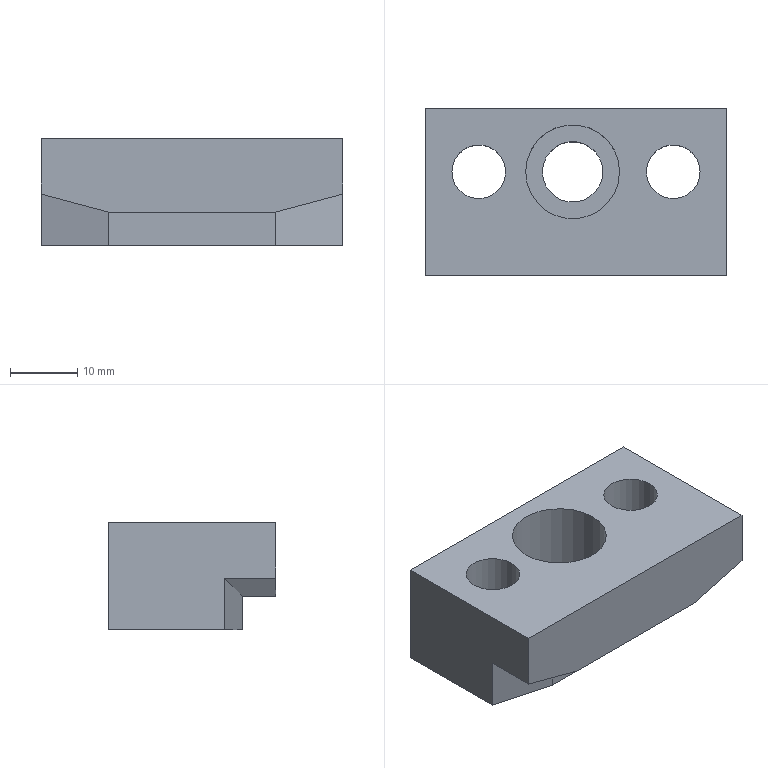Part | STEP file | 1 solid | 17 faces | box 45 x 25 x 16 mm | volume 13030 mm3 | plane 13 | cylinder 4 | commonest cylinder face diameters 8 x2 9 x1 14 x1
STEP:
#1=CARTESIAN_POINT('',(-193.,101.3,3.));
#2=VERTEX_POINT('',#1);
#3=CARTESIAN_POINT('',(-183.,103.98,5.679));
#4=VERTEX_POINT('',#3);
#5=CARTESIAN_POINT('',(-177.77,105.381,7.081));
#6=DIRECTION('',(0.9351,0.2506,0.2506));
#7=VECTOR('',#6,1.);
#8=LINE('',#5,#7);
#9=EDGE_CURVE('',#2,#4,#8,.T.);
#10=ORIENTED_EDGE('',*,*,#9,.T.);
#11=CARTESIAN_POINT('',(-183.,96.3,5.679));
#12=VERTEX_POINT('',#11);
#13=CARTESIAN_POINT('',(-183.,93.8,5.679));
#14=DIRECTION('',(0.,-1.,0.));
#15=VECTOR('',#14,1.);
#16=LINE('',#13,#15);
#17=EDGE_CURVE('',#4,#12,#16,.T.);
#18=ORIENTED_EDGE('',*,*,#17,.T.);
#19=CARTESIAN_POINT('',(-193.,96.3,3.));
#20=VERTEX_POINT('',#19);
#21=CARTESIAN_POINT('',(-185.67,96.3,4.964));
#22=DIRECTION('',(-0.9659,0.,-0.2588));
#23=VECTOR('',#22,1.);
#24=LINE('',#21,#23);
#25=EDGE_CURVE('',#12,#20,#24,.T.);
#26=ORIENTED_EDGE('',*,*,#25,.T.);
#27=CARTESIAN_POINT('',(-193.,101.48,3.));
#28=DIRECTION('',(0.,1.,0.));
#29=VECTOR('',#28,1.);
#30=LINE('',#27,#29);
#31=EDGE_CURVE('',#20,#2,#30,.T.);
#32=ORIENTED_EDGE('',*,*,#31,.T.);
#33=EDGE_LOOP('',(#10,#18,#26,#32));
#34=FACE_OUTER_BOUND('',#33,.T.);
#35=CARTESIAN_POINT('',(-183.,123.8,5.679));
#36=DIRECTION('',(0.2588,0.,-0.9659));
#37=DIRECTION('',(0.9659,0.,0.2588));
#38=AXIS2_PLACEMENT_3D('',#35,#36,#37);
#39=PLANE('',#38);
#40=ADVANCED_FACE('',(#34),#39,.T.);
#41=CARTESIAN_POINT('',(-218.,101.3,3.));
#42=VERTEX_POINT('',#41);
#43=CARTESIAN_POINT('',(-308.,101.3,3.));
#44=DIRECTION('',(-1.,0.,0.));
#45=VECTOR('',#44,1.);
#46=LINE('',#43,#45);
#47=EDGE_CURVE('',#2,#42,#46,.T.);
#48=ORIENTED_EDGE('',*,*,#47,.F.);
#49=ORIENTED_EDGE('',*,*,#31,.F.);
#50=CARTESIAN_POINT('',(-218.,96.3,3.));
#51=VERTEX_POINT('',#50);
#52=CARTESIAN_POINT('',(-218.,96.3,3.));
#53=DIRECTION('',(1.,0.,0.));
#54=VECTOR('',#53,1.);
#55=LINE('',#52,#54);
#56=EDGE_CURVE('',#51,#20,#55,.T.);
#57=ORIENTED_EDGE('',*,*,#56,.F.);
#58=CARTESIAN_POINT('',(-218.,101.48,3.));
#59=DIRECTION('',(0.,1.,0.));
#60=VECTOR('',#59,1.);
#61=LINE('',#58,#60);
#62=EDGE_CURVE('',#51,#42,#61,.T.);
#63=ORIENTED_EDGE('',*,*,#62,.T.);
#64=EDGE_LOOP('',(#48,#49,#57,#63));
#65=FACE_OUTER_BOUND('',#64,.T.);
#66=CARTESIAN_POINT('',(-229.,111.8,3.));
#67=DIRECTION('',(0.,0.,1.));
#68=DIRECTION('',(-1.,0.,0.));
#69=AXIS2_PLACEMENT_3D('',#66,#67,#68);
#70=PLANE('',#69);
#71=ADVANCED_FACE('',(#65),#70,.F.);
#72=CARTESIAN_POINT('',(-228.,103.98,5.679));
#73=VERTEX_POINT('',#72);
#74=CARTESIAN_POINT('',(-233.23,105.381,7.081));
#75=DIRECTION('',(-0.9351,0.2506,0.2506));
#76=VECTOR('',#75,1.);
#77=LINE('',#74,#76);
#78=EDGE_CURVE('',#42,#73,#77,.T.);
#79=ORIENTED_EDGE('',*,*,#78,.F.);
#80=ORIENTED_EDGE('',*,*,#62,.F.);
#81=CARTESIAN_POINT('',(-228.,96.3,5.679));
#82=VERTEX_POINT('',#81);
#83=CARTESIAN_POINT('',(-225.33,96.3,4.964));
#84=DIRECTION('',(0.9659,0.,-0.2588));
#85=VECTOR('',#84,1.);
#86=LINE('',#83,#85);
#87=EDGE_CURVE('',#82,#51,#86,.T.);
#88=ORIENTED_EDGE('',*,*,#87,.F.);
#89=CARTESIAN_POINT('',(-228.,93.8,5.679));
#90=DIRECTION('',(0.,-1.,0.));
#91=VECTOR('',#90,1.);
#92=LINE('',#89,#91);
#93=EDGE_CURVE('',#73,#82,#92,.T.);
#94=ORIENTED_EDGE('',*,*,#93,.F.);
#95=EDGE_LOOP('',(#79,#80,#88,#94));
#96=FACE_OUTER_BOUND('',#95,.T.);
#97=CARTESIAN_POINT('',(-228.,123.8,5.679));
#98=DIRECTION('',(-0.2588,0.,-0.9659));
#99=DIRECTION('',(-0.9659,0.,0.2588));
#100=AXIS2_PLACEMENT_3D('',#97,#98,#99);
#101=PLANE('',#100);
#102=ADVANCED_FACE('',(#96),#101,.T.);
#103=CARTESIAN_POINT('',(-217.998,101.3,-2.));
#104=VERTEX_POINT('',#103);
#105=CARTESIAN_POINT('',(-217.998,101.3,14.));
#106=DIRECTION('',(0.,0.,1.));
#107=VECTOR('',#106,1.);
#108=LINE('',#105,#107);
#109=EDGE_CURVE('',#104,#42,#108,.T.);
#110=ORIENTED_EDGE('',*,*,#109,.T.);
#111=ORIENTED_EDGE('',*,*,#78,.T.);
#112=CARTESIAN_POINT('',(-228.,103.98,-2.));
#113=VERTEX_POINT('',#112);
#114=CARTESIAN_POINT('',(-228.,103.98,-2.));
#115=DIRECTION('',(0.,0.,1.));
#116=VECTOR('',#115,1.);
#117=LINE('',#114,#116);
#118=EDGE_CURVE('',#113,#73,#117,.T.);
#119=ORIENTED_EDGE('',*,*,#118,.F.);
#120=CARTESIAN_POINT('',(-220.317,101.921,-2.));
#121=DIRECTION('',(0.9659,-0.2588,0.));
#122=VECTOR('',#121,1.);
#123=LINE('',#120,#122);
#124=EDGE_CURVE('',#113,#104,#123,.T.);
#125=ORIENTED_EDGE('',*,*,#124,.T.);
#126=EDGE_LOOP('',(#110,#111,#119,#125));
#127=FACE_OUTER_BOUND('',#126,.T.);
#128=CARTESIAN_POINT('',(-218.,101.3,14.));
#129=DIRECTION('',(-0.2588,-0.9659,0.));
#130=DIRECTION('',(0.9659,-0.2588,0.));
#131=AXIS2_PLACEMENT_3D('',#128,#129,#130);
#132=PLANE('',#131);
#133=ADVANCED_FACE('',(#127),#132,.T.);
#134=ORIENTED_EDGE('',*,*,#47,.T.);
#135=ORIENTED_EDGE('',*,*,#109,.F.);
#136=CARTESIAN_POINT('',(-193.002,101.3,-2.));
#137=VERTEX_POINT('',#136);
#138=CARTESIAN_POINT('',(-229.,101.3,-2.));
#139=DIRECTION('',(1.,0.,0.));
#140=VECTOR('',#139,1.);
#141=LINE('',#138,#140);
#142=EDGE_CURVE('',#104,#137,#141,.T.);
#143=ORIENTED_EDGE('',*,*,#142,.T.);
#144=CARTESIAN_POINT('',(-193.002,101.3,14.));
#145=DIRECTION('',(0.,0.,1.));
#146=VECTOR('',#145,1.);
#147=LINE('',#144,#146);
#148=EDGE_CURVE('',#137,#2,#147,.T.);
#149=ORIENTED_EDGE('',*,*,#148,.T.);
#150=EDGE_LOOP('',(#134,#135,#143,#149));
#151=FACE_OUTER_BOUND('',#150,.T.);
#152=CARTESIAN_POINT('',(-308.,101.3,14.));
#153=DIRECTION('',(0.,-1.,0.));
#154=DIRECTION('',(0.,0.,-1.));
#155=AXIS2_PLACEMENT_3D('',#152,#153,#154);
#156=PLANE('',#155);
#157=ADVANCED_FACE('',(#151),#156,.T.);
#158=ORIENTED_EDGE('',*,*,#148,.F.);
#159=CARTESIAN_POINT('',(-183.,103.98,-2.));
#160=VERTEX_POINT('',#159);
#161=CARTESIAN_POINT('',(-190.683,101.921,-2.));
#162=DIRECTION('',(-0.9659,-0.2588,0.));
#163=VECTOR('',#162,1.);
#164=LINE('',#161,#163);
#165=EDGE_CURVE('',#160,#137,#164,.T.);
#166=ORIENTED_EDGE('',*,*,#165,.F.);
#167=CARTESIAN_POINT('',(-183.,103.98,-2.));
#168=DIRECTION('',(0.,0.,1.));
#169=VECTOR('',#168,1.);
#170=LINE('',#167,#169);
#171=EDGE_CURVE('',#160,#4,#170,.T.);
#172=ORIENTED_EDGE('',*,*,#171,.T.);
#173=ORIENTED_EDGE('',*,*,#9,.F.);
#174=EDGE_LOOP('',(#158,#166,#172,#173));
#175=FACE_OUTER_BOUND('',#174,.T.);
#176=CARTESIAN_POINT('',(-193.,101.3,14.));
#177=DIRECTION('',(0.2588,-0.9659,0.));
#178=DIRECTION('',(-0.9659,-0.2588,0.));
#179=AXIS2_PLACEMENT_3D('',#176,#177,#178);
#180=PLANE('',#179);
#181=ADVANCED_FACE('',(#175),#180,.T.);
#182=ORIENTED_EDGE('',*,*,#171,.F.);
#183=CARTESIAN_POINT('',(-183.,121.3,-2.));
#184=VERTEX_POINT('',#183);
#185=CARTESIAN_POINT('',(-183.,123.8,-2.));
#186=DIRECTION('',(0.,-1.,0.));
#187=VECTOR('',#186,1.);
#188=LINE('',#185,#187);
#189=EDGE_CURVE('',#184,#160,#188,.T.);
#190=ORIENTED_EDGE('',*,*,#189,.F.);
#191=CARTESIAN_POINT('',(-183.,121.3,14.));
#192=VERTEX_POINT('',#191);
#193=CARTESIAN_POINT('',(-183.,121.3,-2.));
#194=DIRECTION('',(0.,0.,1.));
#195=VECTOR('',#194,1.);
#196=LINE('',#193,#195);
#197=EDGE_CURVE('',#184,#192,#196,.T.);
#198=ORIENTED_EDGE('',*,*,#197,.T.);
#199=CARTESIAN_POINT('',(-183.,96.3,14.));
#200=VERTEX_POINT('',#199);
#201=CARTESIAN_POINT('',(-183.,123.8,14.));
#202=DIRECTION('',(0.,-1.,0.));
#203=VECTOR('',#202,1.);
#204=LINE('',#201,#203);
#205=EDGE_CURVE('',#192,#200,#204,.T.);
#206=ORIENTED_EDGE('',*,*,#205,.T.);
#207=CARTESIAN_POINT('',(-183.,96.3,-2.));
#208=DIRECTION('',(0.,0.,1.));
#209=VECTOR('',#208,1.);
#210=LINE('',#207,#209);
#211=EDGE_CURVE('',#12,#200,#210,.T.);
#212=ORIENTED_EDGE('',*,*,#211,.F.);
#213=ORIENTED_EDGE('',*,*,#17,.F.);
#214=EDGE_LOOP('',(#182,#190,#198,#206,#212,#213));
#215=FACE_OUTER_BOUND('',#214,.T.);
#216=CARTESIAN_POINT('',(-183.,123.8,-2.));
#217=DIRECTION('',(1.,0.,0.));
#218=DIRECTION('',(0.,0.,1.));
#219=AXIS2_PLACEMENT_3D('',#216,#217,#218);
#220=PLANE('',#219);
#221=ADVANCED_FACE('',(#215),#220,.T.);
#222=CARTESIAN_POINT('',(-228.,96.3,14.));
#223=VERTEX_POINT('',#222);
#224=CARTESIAN_POINT('',(-218.,96.3,14.));
#225=DIRECTION('',(1.,0.,0.));
#226=VECTOR('',#225,1.);
#227=LINE('',#224,#226);
#228=EDGE_CURVE('',#223,#200,#227,.T.);
#229=ORIENTED_EDGE('',*,*,#228,.F.);
#230=CARTESIAN_POINT('',(-228.,96.3,-2.));
#231=DIRECTION('',(0.,0.,1.));
#232=VECTOR('',#231,1.);
#233=LINE('',#230,#232);
#234=EDGE_CURVE('',#82,#223,#233,.T.);
#235=ORIENTED_EDGE('',*,*,#234,.F.);
#236=ORIENTED_EDGE('',*,*,#87,.T.);
#237=ORIENTED_EDGE('',*,*,#56,.T.);
#238=ORIENTED_EDGE('',*,*,#25,.F.);
#239=ORIENTED_EDGE('',*,*,#211,.T.);
#240=EDGE_LOOP('',(#229,#235,#236,#237,#238,#239));
#241=FACE_OUTER_BOUND('',#240,.T.);
#242=CARTESIAN_POINT('',(-218.,96.3,-2.));
#243=DIRECTION('',(0.,-1.,0.));
#244=DIRECTION('',(0.,0.,-1.));
#245=AXIS2_PLACEMENT_3D('',#242,#243,#244);
#246=PLANE('',#245);
#247=ADVANCED_FACE('',(#241),#246,.T.);
#248=ORIENTED_EDGE('',*,*,#118,.T.);
#249=ORIENTED_EDGE('',*,*,#93,.T.);
#250=ORIENTED_EDGE('',*,*,#234,.T.);
#251=CARTESIAN_POINT('',(-228.,121.3,14.));
#252=VERTEX_POINT('',#251);
#253=CARTESIAN_POINT('',(-228.,123.8,14.));
#254=DIRECTION('',(0.,-1.,0.));
#255=VECTOR('',#254,1.);
#256=LINE('',#253,#255);
#257=EDGE_CURVE('',#252,#223,#256,.T.);
#258=ORIENTED_EDGE('',*,*,#257,.F.);
#259=CARTESIAN_POINT('',(-228.,121.3,-2.));
#260=VERTEX_POINT('',#259);
#261=CARTESIAN_POINT('',(-228.,121.3,-2.));
#262=DIRECTION('',(0.,0.,1.));
#263=VECTOR('',#262,1.);
#264=LINE('',#261,#263);
#265=EDGE_CURVE('',#260,#252,#264,.T.);
#266=ORIENTED_EDGE('',*,*,#265,.F.);
#267=CARTESIAN_POINT('',(-228.,123.8,-2.));
#268=DIRECTION('',(0.,-1.,0.));
#269=VECTOR('',#268,1.);
#270=LINE('',#267,#269);
#271=EDGE_CURVE('',#260,#113,#270,.T.);
#272=ORIENTED_EDGE('',*,*,#271,.T.);
#273=EDGE_LOOP('',(#248,#249,#250,#258,#266,#272));
#274=FACE_OUTER_BOUND('',#273,.T.);
#275=CARTESIAN_POINT('',(-228.,123.8,-2.));
#276=DIRECTION('',(-1.,0.,0.));
#277=DIRECTION('',(0.,0.,1.));
#278=AXIS2_PLACEMENT_3D('',#275,#276,#277);
#279=PLANE('',#278);
#280=ADVANCED_FACE('',(#274),#279,.T.);
#281=CARTESIAN_POINT('',(-229.,121.3,-2.));
#282=DIRECTION('',(-1.,0.,0.));
#283=VECTOR('',#282,1.);
#284=LINE('',#281,#283);
#285=EDGE_CURVE('',#184,#260,#284,.T.);
#286=ORIENTED_EDGE('',*,*,#285,.T.);
#287=ORIENTED_EDGE('',*,*,#265,.T.);
#288=CARTESIAN_POINT('',(-229.,121.3,14.));
#289=DIRECTION('',(-1.,0.,0.));
#290=VECTOR('',#289,1.);
#291=LINE('',#288,#290);
#292=EDGE_CURVE('',#192,#252,#291,.T.);
#293=ORIENTED_EDGE('',*,*,#292,.F.);
#294=ORIENTED_EDGE('',*,*,#197,.F.);
#295=EDGE_LOOP('',(#286,#287,#293,#294));
#296=FACE_OUTER_BOUND('',#295,.T.);
#297=CARTESIAN_POINT('',(-318.,121.3,-2.));
#298=DIRECTION('',(0.,1.,0.));
#299=DIRECTION('',(0.,0.,1.));
#300=AXIS2_PLACEMENT_3D('',#297,#298,#299);
#301=PLANE('',#300);
#302=ADVANCED_FACE('',(#296),#301,.T.);
#303=CARTESIAN_POINT('',(-224.,111.8,14.));
#304=VERTEX_POINT('',#303);
#305=CARTESIAN_POINT('',(-220.,111.8,14.));
#306=DIRECTION('',(0.,0.,1.));
#307=DIRECTION('',(-1.,0.,0.));
#308=AXIS2_PLACEMENT_3D('',#305,#306,#307);
#309=CIRCLE('',#308,4.);
#310=EDGE_CURVE('',#304,#304,#309,.T.);
#311=ORIENTED_EDGE('',*,*,#310,.F.);
#312=EDGE_LOOP('',(#311));
#313=FACE_BOUND('',#312,.T.);
#314=CARTESIAN_POINT('',(-199.,111.8,14.));
#315=VERTEX_POINT('',#314);
#316=CARTESIAN_POINT('',(-206.,111.8,14.));
#317=DIRECTION('',(0.,0.,-1.));
#318=DIRECTION('',(1.,0.,0.));
#319=AXIS2_PLACEMENT_3D('',#316,#317,#318);
#320=CIRCLE('',#319,7.);
#321=EDGE_CURVE('',#315,#315,#320,.T.);
#322=ORIENTED_EDGE('',*,*,#321,.T.);
#323=EDGE_LOOP('',(#322));
#324=FACE_BOUND('',#323,.T.);
#325=CARTESIAN_POINT('',(-187.,111.8,14.));
#326=VERTEX_POINT('',#325);
#327=CARTESIAN_POINT('',(-191.,111.8,14.));
#328=DIRECTION('',(0.,0.,-1.));
#329=DIRECTION('',(1.,0.,0.));
#330=AXIS2_PLACEMENT_3D('',#327,#328,#329);
#331=CIRCLE('',#330,4.);
#332=EDGE_CURVE('',#326,#326,#331,.T.);
#333=ORIENTED_EDGE('',*,*,#332,.T.);
#334=EDGE_LOOP('',(#333));
#335=FACE_BOUND('',#334,.T.);
#336=ORIENTED_EDGE('',*,*,#292,.T.);
#337=ORIENTED_EDGE('',*,*,#257,.T.);
#338=ORIENTED_EDGE('',*,*,#228,.T.);
#339=ORIENTED_EDGE('',*,*,#205,.F.);
#340=EDGE_LOOP('',(#336,#337,#338,#339));
#341=FACE_BOUND('',#340,.T.);
#342=CARTESIAN_POINT('',(-229.,111.8,14.));
#343=DIRECTION('',(0.,0.,1.));
#344=DIRECTION('',(-1.,0.,0.));
#345=AXIS2_PLACEMENT_3D('',#342,#343,#344);
#346=PLANE('',#345);
#347=ADVANCED_FACE('',(#313,#324,#335,#341),#346,.T.);
#348=CARTESIAN_POINT('',(-224.,111.8,-2.));
#349=VERTEX_POINT('',#348);
#350=CARTESIAN_POINT('',(-220.,111.8,-2.));
#351=DIRECTION('',(0.,0.,-1.));
#352=DIRECTION('',(-1.,0.,0.));
#353=AXIS2_PLACEMENT_3D('',#350,#351,#352);
#354=CIRCLE('',#353,4.);
#355=EDGE_CURVE('',#349,#349,#354,.T.);
#356=ORIENTED_EDGE('',*,*,#355,.F.);
#357=EDGE_LOOP('',(#356));
#358=FACE_BOUND('',#357,.T.);
#359=CARTESIAN_POINT('',(-201.5,111.8,-2.));
#360=VERTEX_POINT('',#359);
#361=CARTESIAN_POINT('',(-206.,111.8,-2.));
#362=DIRECTION('',(0.,0.,1.));
#363=DIRECTION('',(1.,0.,0.));
#364=AXIS2_PLACEMENT_3D('',#361,#362,#363);
#365=CIRCLE('',#364,4.5);
#366=EDGE_CURVE('',#360,#360,#365,.T.);
#367=ORIENTED_EDGE('',*,*,#366,.T.);
#368=EDGE_LOOP('',(#367));
#369=FACE_BOUND('',#368,.T.);
#370=CARTESIAN_POINT('',(-187.,111.8,-2.));
#371=VERTEX_POINT('',#370);
#372=CARTESIAN_POINT('',(-191.,111.8,-2.));
#373=DIRECTION('',(0.,0.,1.));
#374=DIRECTION('',(1.,0.,0.));
#375=AXIS2_PLACEMENT_3D('',#372,#373,#374);
#376=CIRCLE('',#375,4.);
#377=EDGE_CURVE('',#371,#371,#376,.T.);
#378=ORIENTED_EDGE('',*,*,#377,.T.);
#379=EDGE_LOOP('',(#378));
#380=FACE_BOUND('',#379,.T.);
#381=ORIENTED_EDGE('',*,*,#285,.F.);
#382=ORIENTED_EDGE('',*,*,#189,.T.);
#383=ORIENTED_EDGE('',*,*,#165,.T.);
#384=ORIENTED_EDGE('',*,*,#142,.F.);
#385=ORIENTED_EDGE('',*,*,#124,.F.);
#386=ORIENTED_EDGE('',*,*,#271,.F.);
#387=EDGE_LOOP('',(#381,#382,#383,#384,#385,#386));
#388=FACE_BOUND('',#387,.T.);
#389=CARTESIAN_POINT('',(-229.,111.8,-2.));
#390=DIRECTION('',(0.,0.,1.));
#391=DIRECTION('',(-1.,0.,0.));
#392=AXIS2_PLACEMENT_3D('',#389,#390,#391);
#393=PLANE('',#392);
#394=ADVANCED_FACE('',(#358,#369,#380,#388),#393,.F.);
#395=ORIENTED_EDGE('',*,*,#332,.F.);
#396=EDGE_LOOP('',(#395));
#397=FACE_BOUND('',#396,.T.);
#398=ORIENTED_EDGE('',*,*,#377,.F.);
#399=EDGE_LOOP('',(#398));
#400=FACE_BOUND('',#399,.T.);
#401=CARTESIAN_POINT('',(-191.,111.8,-2.));
#402=DIRECTION('',(0.,0.,1.));
#403=DIRECTION('',(1.,0.,0.));
#404=AXIS2_PLACEMENT_3D('',#401,#402,#403);
#405=CYLINDRICAL_SURFACE('',#404,4.);
#406=ADVANCED_FACE('',(#397,#400),#405,.F.);
#407=CARTESIAN_POINT('',(-210.5,111.8,4.));
#408=VERTEX_POINT('',#407);
#409=CARTESIAN_POINT('',(-206.,111.8,4.));
#410=DIRECTION('',(0.,0.,-1.));
#411=DIRECTION('',(-1.,0.,0.));
#412=AXIS2_PLACEMENT_3D('',#409,#410,#411);
#413=CIRCLE('',#412,4.5);
#414=EDGE_CURVE('',#408,#408,#413,.T.);
#415=ORIENTED_EDGE('',*,*,#414,.F.);
#416=EDGE_LOOP('',(#415));
#417=FACE_BOUND('',#416,.T.);
#418=ORIENTED_EDGE('',*,*,#366,.F.);
#419=EDGE_LOOP('',(#418));
#420=FACE_BOUND('',#419,.T.);
#421=CARTESIAN_POINT('',(-206.,111.8,-2.));
#422=DIRECTION('',(0.,0.,1.));
#423=DIRECTION('',(1.,0.,0.));
#424=AXIS2_PLACEMENT_3D('',#421,#422,#423);
#425=CYLINDRICAL_SURFACE('',#424,4.5);
#426=ADVANCED_FACE('',(#417,#420),#425,.F.);
#427=ORIENTED_EDGE('',*,*,#414,.T.);
#428=EDGE_LOOP('',(#427));
#429=FACE_BOUND('',#428,.T.);
#430=CARTESIAN_POINT('',(-199.,111.8,4.));
#431=VERTEX_POINT('',#430);
#432=CARTESIAN_POINT('',(-206.,111.8,4.));
#433=DIRECTION('',(0.,0.,-1.));
#434=DIRECTION('',(1.,0.,0.));
#435=AXIS2_PLACEMENT_3D('',#432,#433,#434);
#436=CIRCLE('',#435,7.);
#437=EDGE_CURVE('',#431,#431,#436,.T.);
#438=ORIENTED_EDGE('',*,*,#437,.F.);
#439=EDGE_LOOP('',(#438));
#440=FACE_BOUND('',#439,.T.);
#441=CARTESIAN_POINT('',(-206.,111.8,4.));
#442=DIRECTION('',(0.,0.,-1.));
#443=DIRECTION('',(-1.,0.,0.));
#444=AXIS2_PLACEMENT_3D('',#441,#442,#443);
#445=PLANE('',#444);
#446=ADVANCED_FACE('',(#429,#440),#445,.F.);
#447=ORIENTED_EDGE('',*,*,#321,.F.);
#448=EDGE_LOOP('',(#447));
#449=FACE_BOUND('',#448,.T.);
#450=ORIENTED_EDGE('',*,*,#437,.T.);
#451=EDGE_LOOP('',(#450));
#452=FACE_BOUND('',#451,.T.);
#453=CARTESIAN_POINT('',(-206.,111.8,4.));
#454=DIRECTION('',(0.,0.,1.));
#455=DIRECTION('',(1.,0.,0.));
#456=AXIS2_PLACEMENT_3D('',#453,#454,#455);
#457=CYLINDRICAL_SURFACE('',#456,7.);
#458=ADVANCED_FACE('',(#449,#452),#457,.F.);
#459=ORIENTED_EDGE('',*,*,#310,.T.);
#460=EDGE_LOOP('',(#459));
#461=FACE_BOUND('',#460,.T.);
#462=ORIENTED_EDGE('',*,*,#355,.T.);
#463=EDGE_LOOP('',(#462));
#464=FACE_BOUND('',#463,.T.);
#465=CARTESIAN_POINT('',(-220.,111.8,-2.));
#466=DIRECTION('',(0.,0.,1.));
#467=DIRECTION('',(-1.,0.,0.));
#468=AXIS2_PLACEMENT_3D('',#465,#466,#467);
#469=CYLINDRICAL_SURFACE('',#468,4.);
#470=ADVANCED_FACE('',(#461,#464),#469,.F.);
#471=CLOSED_SHELL('',(#40,#71,#102,#133,#157,#181,#221,#247,#280,#302,#347,#394,#406,#426,#446,#458,#470));
#472=MANIFOLD_SOLID_BREP('',#471);
#473=(LENGTH_UNIT()NAMED_UNIT(*)SI_UNIT(.MILLI.,.METRE.));
#474=UNCERTAINTY_MEASURE_WITH_UNIT(LENGTH_MEASURE(0.002713),#473,'','');
#475=(NAMED_UNIT(*)PLANE_ANGLE_UNIT()SI_UNIT($,.RADIAN.));
#476=PLANE_ANGLE_MEASURE_WITH_UNIT(PLANE_ANGLE_MEASURE(0.01745),#475);
#477=DIMENSIONAL_EXPONENTS(0.,0.,0.,0.,0.,0.,0.);
#478=(CONVERSION_BASED_UNIT('DEGREE',#476)NAMED_UNIT(#477)PLANE_ANGLE_UNIT());
#479=(NAMED_UNIT(*)SI_UNIT($,.STERADIAN.)SOLID_ANGLE_UNIT());
#480=(GEOMETRIC_REPRESENTATION_CONTEXT(3)GLOBAL_UNCERTAINTY_ASSIGNED_CONTEXT((#474))GLOBAL_UNIT_ASSIGNED_CONTEXT((#473,#478,#479))REPRESENTATION_CONTEXT('',''));
#481=ADVANCED_BREP_SHAPE_REPRESENTATION('',(#472),#480);